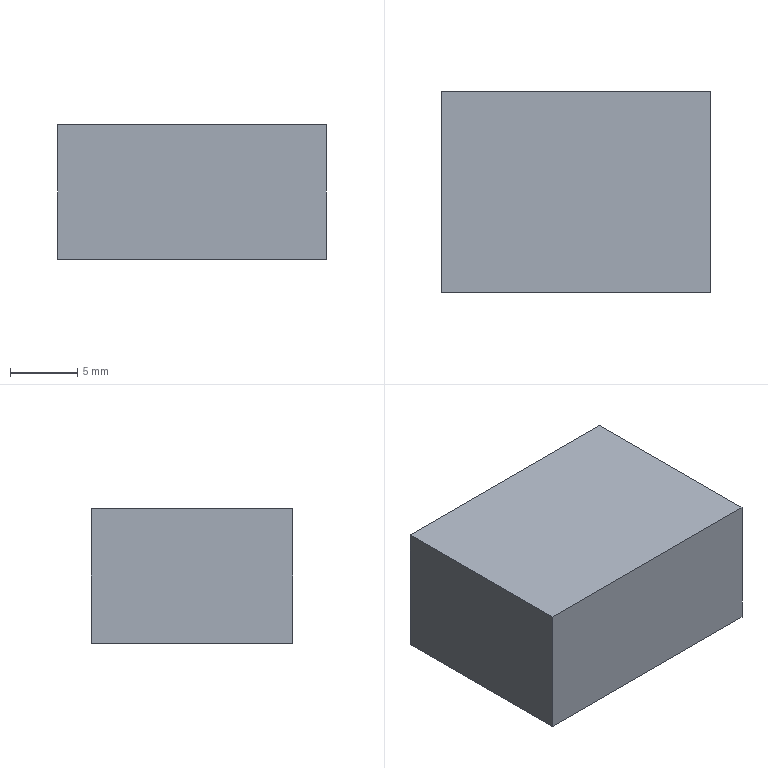Part | SolidWorks | features Extrusion 1 | 1 solid | 6 faces | box 20 x 15 x 10 mm | volume 3000 mm3 | plane 6
STEP:
#1=CARTESIAN_POINT('',(0.,0.,-10.));
#2=VERTEX_POINT('',#1);
#3=CARTESIAN_POINT('',(0.,0.,0.));
#4=VERTEX_POINT('',#3);
#5=CARTESIAN_POINT('',(0.,0.,0.));
#6=DIRECTION('',(0.,0.,1.));
#7=VECTOR('',#6,1000.);
#8=LINE('',#5,#7);
#9=EDGE_CURVE('',#2,#4,#8,.T.);
#10=ORIENTED_EDGE('',*,*,#9,.T.);
#11=CARTESIAN_POINT('',(0.,15.,0.));
#12=VERTEX_POINT('',#11);
#13=CARTESIAN_POINT('',(0.,15.,0.));
#14=DIRECTION('',(0.,-1.,0.));
#15=VECTOR('',#14,1000.);
#16=LINE('',#13,#15);
#17=EDGE_CURVE('',#12,#4,#16,.T.);
#18=ORIENTED_EDGE('',*,*,#17,.F.);
#19=CARTESIAN_POINT('',(0.,15.,-10.));
#20=VERTEX_POINT('',#19);
#21=CARTESIAN_POINT('',(0.,15.,0.));
#22=DIRECTION('',(0.,0.,1.));
#23=VECTOR('',#22,1000.);
#24=LINE('',#21,#23);
#25=EDGE_CURVE('',#20,#12,#24,.T.);
#26=ORIENTED_EDGE('',*,*,#25,.F.);
#27=CARTESIAN_POINT('',(0.,15.,-10.));
#28=DIRECTION('',(0.,-1.,0.));
#29=VECTOR('',#28,1000.);
#30=LINE('',#27,#29);
#31=EDGE_CURVE('',#20,#2,#30,.T.);
#32=ORIENTED_EDGE('',*,*,#31,.T.);
#33=EDGE_LOOP('',(#10,#18,#26,#32));
#34=FACE_OUTER_BOUND('',#33,.T.);
#35=CARTESIAN_POINT('',(0.,15.,0.));
#36=DIRECTION('',(1.,0.,0.));
#37=DIRECTION('',(0.,0.,-1.));
#38=AXIS2_PLACEMENT_3D('',#35,#36,#37);
#39=PLANE('',#38);
#40=ADVANCED_FACE('',(#34),#39,.F.);
#41=CARTESIAN_POINT('',(20.,0.,0.));
#42=VERTEX_POINT('',#41);
#43=CARTESIAN_POINT('',(0.,0.,0.));
#44=DIRECTION('',(1.,0.,0.));
#45=VECTOR('',#44,1000.);
#46=LINE('',#43,#45);
#47=EDGE_CURVE('',#4,#42,#46,.T.);
#48=ORIENTED_EDGE('',*,*,#47,.T.);
#49=CARTESIAN_POINT('',(20.,15.,0.));
#50=VERTEX_POINT('',#49);
#51=CARTESIAN_POINT('',(20.,15.,0.));
#52=DIRECTION('',(0.,-1.,0.));
#53=VECTOR('',#52,1000.);
#54=LINE('',#51,#53);
#55=EDGE_CURVE('',#50,#42,#54,.T.);
#56=ORIENTED_EDGE('',*,*,#55,.F.);
#57=CARTESIAN_POINT('',(0.,15.,0.));
#58=DIRECTION('',(1.,0.,0.));
#59=VECTOR('',#58,1000.);
#60=LINE('',#57,#59);
#61=EDGE_CURVE('',#12,#50,#60,.T.);
#62=ORIENTED_EDGE('',*,*,#61,.F.);
#63=ORIENTED_EDGE('',*,*,#17,.T.);
#64=EDGE_LOOP('',(#48,#56,#62,#63));
#65=FACE_OUTER_BOUND('',#64,.T.);
#66=CARTESIAN_POINT('',(0.,15.,0.));
#67=DIRECTION('',(0.,0.,-1.));
#68=DIRECTION('',(-1.,0.,0.));
#69=AXIS2_PLACEMENT_3D('',#66,#67,#68);
#70=PLANE('',#69);
#71=ADVANCED_FACE('',(#65),#70,.F.);
#72=CARTESIAN_POINT('',(20.,0.,-10.));
#73=VERTEX_POINT('',#72);
#74=CARTESIAN_POINT('',(20.,0.,0.));
#75=DIRECTION('',(0.,0.,-1.));
#76=VECTOR('',#75,1000.);
#77=LINE('',#74,#76);
#78=EDGE_CURVE('',#42,#73,#77,.T.);
#79=ORIENTED_EDGE('',*,*,#78,.T.);
#80=CARTESIAN_POINT('',(20.,15.,-10.));
#81=VERTEX_POINT('',#80);
#82=CARTESIAN_POINT('',(20.,15.,-10.));
#83=DIRECTION('',(0.,-1.,0.));
#84=VECTOR('',#83,1000.);
#85=LINE('',#82,#84);
#86=EDGE_CURVE('',#81,#73,#85,.T.);
#87=ORIENTED_EDGE('',*,*,#86,.F.);
#88=CARTESIAN_POINT('',(20.,15.,0.));
#89=DIRECTION('',(0.,0.,-1.));
#90=VECTOR('',#89,1000.);
#91=LINE('',#88,#90);
#92=EDGE_CURVE('',#50,#81,#91,.T.);
#93=ORIENTED_EDGE('',*,*,#92,.F.);
#94=ORIENTED_EDGE('',*,*,#55,.T.);
#95=EDGE_LOOP('',(#79,#87,#93,#94));
#96=FACE_OUTER_BOUND('',#95,.T.);
#97=CARTESIAN_POINT('',(20.,15.,0.));
#98=DIRECTION('',(-1.,0.,0.));
#99=DIRECTION('',(0.,0.,1.));
#100=AXIS2_PLACEMENT_3D('',#97,#98,#99);
#101=PLANE('',#100);
#102=ADVANCED_FACE('',(#96),#101,.F.);
#103=CARTESIAN_POINT('',(0.,0.,-10.));
#104=DIRECTION('',(-1.,0.,0.));
#105=VECTOR('',#104,1000.);
#106=LINE('',#103,#105);
#107=EDGE_CURVE('',#73,#2,#106,.T.);
#108=ORIENTED_EDGE('',*,*,#107,.T.);
#109=ORIENTED_EDGE('',*,*,#31,.F.);
#110=CARTESIAN_POINT('',(0.,15.,-10.));
#111=DIRECTION('',(-1.,0.,0.));
#112=VECTOR('',#111,1000.);
#113=LINE('',#110,#112);
#114=EDGE_CURVE('',#81,#20,#113,.T.);
#115=ORIENTED_EDGE('',*,*,#114,.F.);
#116=ORIENTED_EDGE('',*,*,#86,.T.);
#117=EDGE_LOOP('',(#108,#109,#115,#116));
#118=FACE_OUTER_BOUND('',#117,.T.);
#119=CARTESIAN_POINT('',(0.,15.,-10.));
#120=DIRECTION('',(0.,0.,1.));
#121=DIRECTION('',(1.,0.,0.));
#122=AXIS2_PLACEMENT_3D('',#119,#120,#121);
#123=PLANE('',#122);
#124=ADVANCED_FACE('',(#118),#123,.F.);
#125=ORIENTED_EDGE('',*,*,#25,.T.);
#126=ORIENTED_EDGE('',*,*,#61,.T.);
#127=ORIENTED_EDGE('',*,*,#92,.T.);
#128=ORIENTED_EDGE('',*,*,#114,.T.);
#129=EDGE_LOOP('',(#125,#126,#127,#128));
#130=FACE_OUTER_BOUND('',#129,.T.);
#131=CARTESIAN_POINT('',(0.,15.,0.));
#132=DIRECTION('',(0.,-1.,0.));
#133=DIRECTION('',(0.,0.,-1.));
#134=AXIS2_PLACEMENT_3D('',#131,#132,#133);
#135=PLANE('',#134);
#136=ADVANCED_FACE('',(#130),#135,.F.);
#137=ORIENTED_EDGE('',*,*,#9,.F.);
#138=ORIENTED_EDGE('',*,*,#107,.F.);
#139=ORIENTED_EDGE('',*,*,#78,.F.);
#140=ORIENTED_EDGE('',*,*,#47,.F.);
#141=EDGE_LOOP('',(#137,#138,#139,#140));
#142=FACE_OUTER_BOUND('',#141,.T.);
#143=CARTESIAN_POINT('',(0.,0.,0.));
#144=DIRECTION('',(0.,-1.,0.));
#145=DIRECTION('',(0.,0.,-1.));
#146=AXIS2_PLACEMENT_3D('',#143,#144,#145);
#147=PLANE('',#146);
#148=ADVANCED_FACE('',(#142),#147,.T.);
#149=CLOSED_SHELL('',(#40,#71,#102,#124,#136,#148));
#150=MANIFOLD_SOLID_BREP('',#149);
#151=CARTESIAN_POINT('',(0.,0.,0.));
#152=DIRECTION('',(0.,0.,1.));
#153=DIRECTION('',(1.,0.,0.));
#154=AXIS2_PLACEMENT_3D('',#151,#152,#153);
#155=(LENGTH_UNIT()NAMED_UNIT(*)SI_UNIT(.MILLI.,.METRE.));
#156=UNCERTAINTY_MEASURE_WITH_UNIT(LENGTH_MEASURE(0.00001),#155,'','');
#157=(NAMED_UNIT(*)PLANE_ANGLE_UNIT()SI_UNIT($,.RADIAN.));
#158=(NAMED_UNIT(*)SI_UNIT($,.STERADIAN.)SOLID_ANGLE_UNIT());
#159=(GEOMETRIC_REPRESENTATION_CONTEXT(3)GLOBAL_UNCERTAINTY_ASSIGNED_CONTEXT((#156))GLOBAL_UNIT_ASSIGNED_CONTEXT((#155,#157,#158))REPRESENTATION_CONTEXT('',''));
#160=ADVANCED_BREP_SHAPE_REPRESENTATION('',(#150,#154),#159);